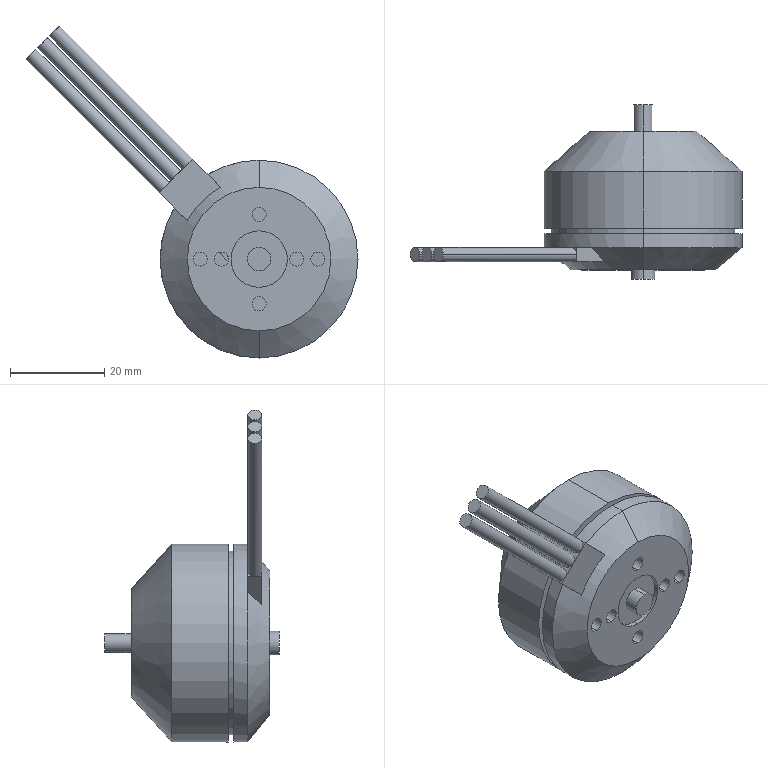Part | SolidWorks | features BaseBody 1 | 1 solid | 78 faces | box 70.497 x 37.1 x 70.497 mm | volume 35098 mm3 | cylinder 40 | plane 34 | cone 4 | commonest cylinder face diameters 3 x26 5 x4 42 x4 4 x2 12 x2 39 x2